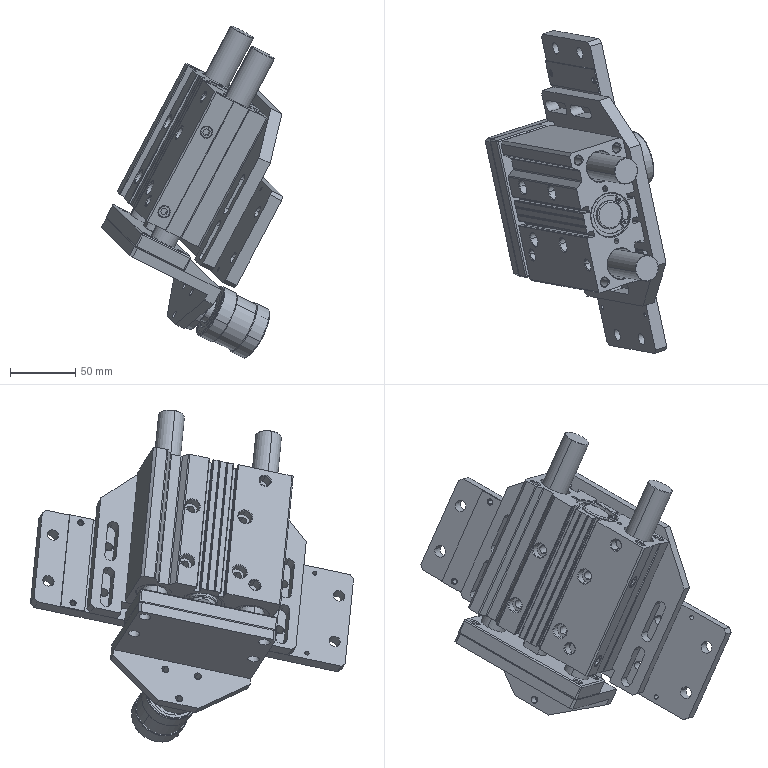Part | SolidWorks | 12 solids | 945 faces | box 139.525 x 248.451 x 255.389 mm | volume 1113097 mm3 | cylinder 350 | plane 273 | cone 124 | torus 112 | sphere 64 | spline 22 | commonest cylinder face diameters 0.4 x34 9 x30 0.8 x28 6.647 x26 4 x18 20 x18